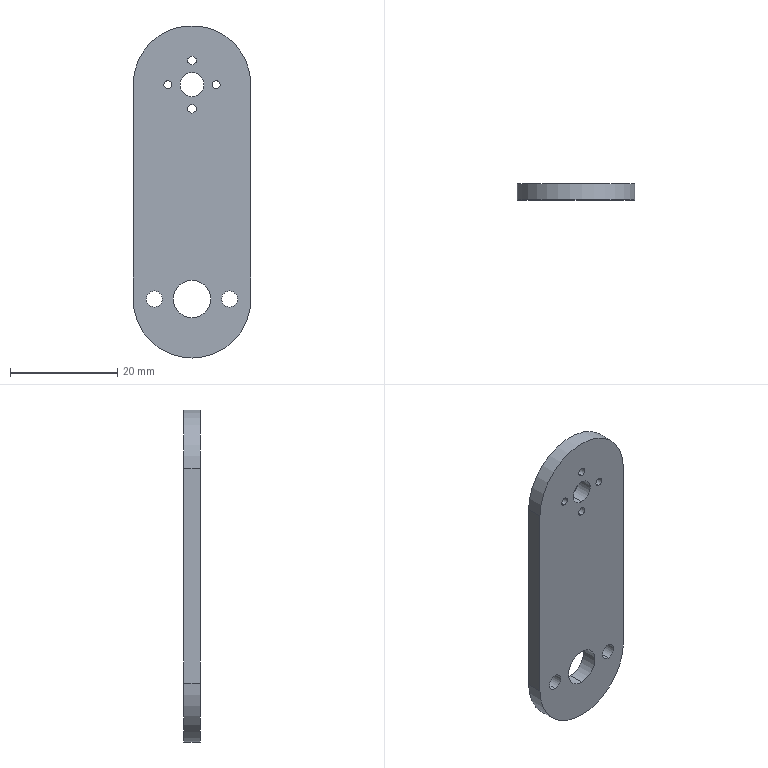Part | STEP file | Dial wheel bracket | 1 solid | 23 faces | box 22 x 3 x 62 mm | volume 3552 mm3 | cylinder 19 | plane 4 | commonest cylinder face diameters 1.5 x4 1.6 x4 3 x4 22 x3 4.5 x2 7 x2